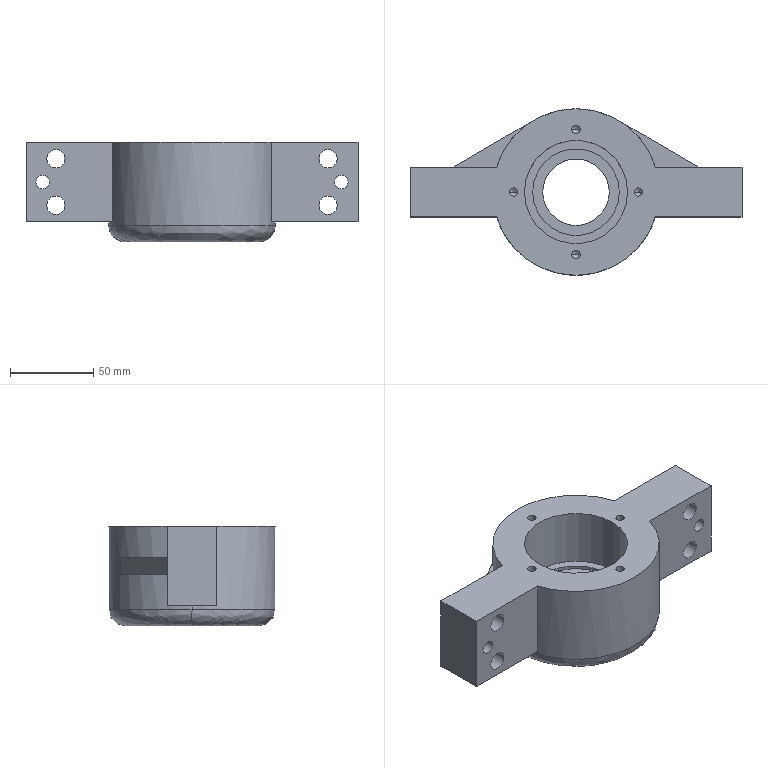Part | STEP file | 45Z Bearing Seat | 1 solid | 71 faces | box 199.394 x 100 x 60 mm | volume 453459 mm3 | cylinder 38 | plane 23 | cone 8 | spline 2 | commonest cylinder face diameters 5 x8 11 x8 8 x4 16 x4 17 x4 52 x4